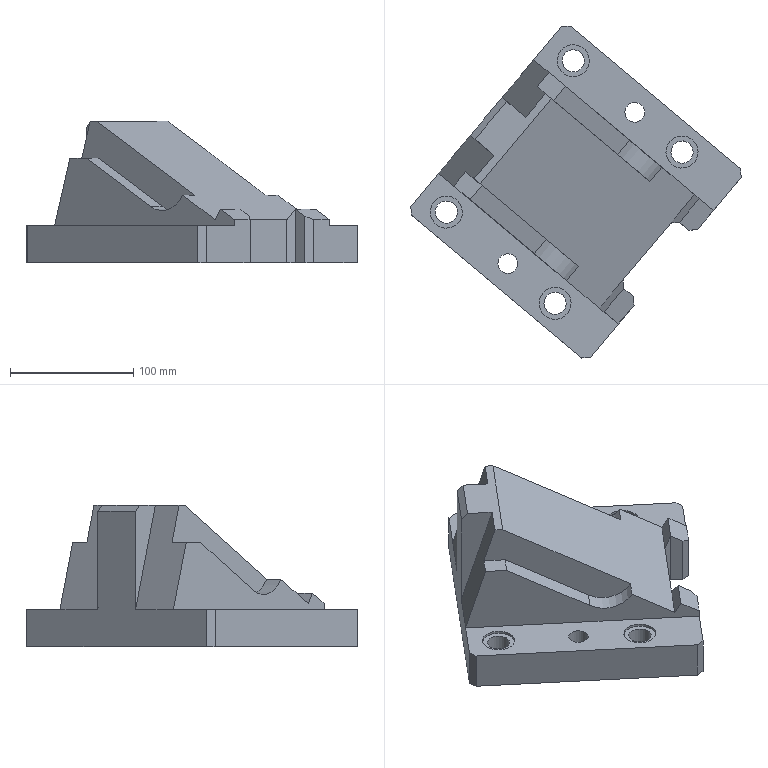Part | NX | features solid 2 | 1 solid | 75 faces | box 267.678 x 268.911 x 115 mm | volume 1899099 mm3 | plane 63 | cylinder 12 | commonest cylinder face diameters 18 x4 26 x4 16 x2 50 x2